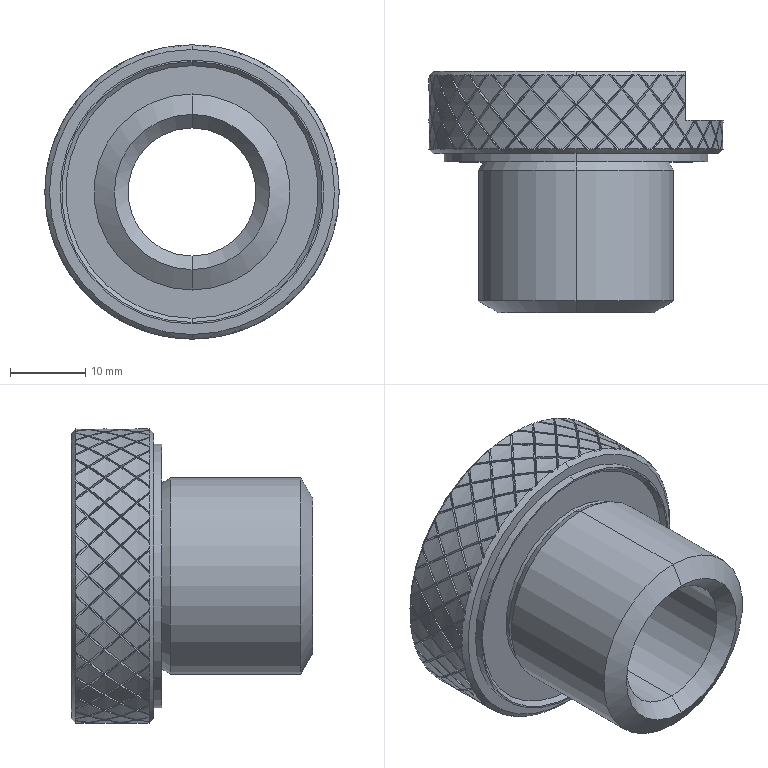Part | SolidWorks | features Chamfer 2, BlendCut 1, CirPattern 1, ICE 1, MirrorPattern 1, Revolution 1 | 1 solid | 1250 faces | box 39 x 32 x 39 mm | volume 16208 mm3 | spline 1058 | cylinder 171 | cone 15 | plane 6 | commonest cylinder face diameters 39 x163 17 x2 24.7 x2 26 x2 35 x2